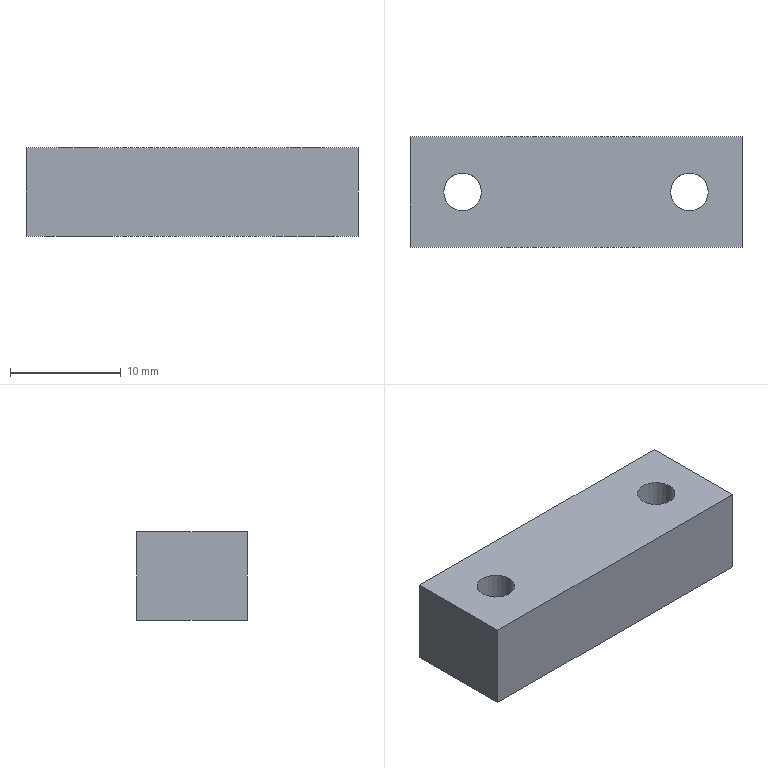Part | SolidWorks | features Extrusion 1, HoleWzd 1 | 1 solid | 16 faces | box 30 x 10 x 8 mm | volume 2124 mm3 | cylinder 8 | plane 8 | commonest cylinder face diameters 3.4 x4 6 x4
STEP:
#1=CARTESIAN_POINT('',(13.25,0.,3.4));
#2=VERTEX_POINT('',#1);
#3=CARTESIAN_POINT('',(7.25,0.,3.4));
#4=VERTEX_POINT('',#3);
#5=CARTESIAN_POINT('',(10.25,0.,3.4));
#6=DIRECTION('',(0.,0.,-1.));
#7=DIRECTION('',(-1.,0.,0.));
#8=AXIS2_PLACEMENT_3D('',#5,#6,#7);
#9=CIRCLE('',#8,3.);
#10=EDGE_CURVE('',#2,#4,#9,.T.);
#11=ORIENTED_EDGE('',*,*,#10,.F.);
#12=CARTESIAN_POINT('',(13.25,0.,0.));
#13=VERTEX_POINT('',#12);
#14=CARTESIAN_POINT('',(13.25,0.,0.));
#15=DIRECTION('',(0.,0.,-1.));
#16=VECTOR('',#15,1000.);
#17=LINE('',#14,#16);
#18=EDGE_CURVE('',#2,#13,#17,.T.);
#19=ORIENTED_EDGE('',*,*,#18,.T.);
#20=CARTESIAN_POINT('',(7.25,0.,0.));
#21=VERTEX_POINT('',#20);
#22=CARTESIAN_POINT('',(10.25,0.,0.));
#23=DIRECTION('',(0.,0.,-1.));
#24=DIRECTION('',(-1.,0.,0.));
#25=AXIS2_PLACEMENT_3D('',#22,#23,#24);
#26=CIRCLE('',#25,3.);
#27=EDGE_CURVE('',#13,#21,#26,.T.);
#28=ORIENTED_EDGE('',*,*,#27,.T.);
#29=CARTESIAN_POINT('',(7.25,0.,0.));
#30=DIRECTION('',(0.,0.,-1.));
#31=VECTOR('',#30,1000.);
#32=LINE('',#29,#31);
#33=EDGE_CURVE('',#4,#21,#32,.T.);
#34=ORIENTED_EDGE('',*,*,#33,.F.);
#35=EDGE_LOOP('',(#11,#19,#28,#34));
#36=FACE_OUTER_BOUND('',#35,.T.);
#37=CARTESIAN_POINT('',(10.25,0.,0.));
#38=DIRECTION('',(0.,0.,-1.));
#39=DIRECTION('',(-1.,0.,0.));
#40=AXIS2_PLACEMENT_3D('',#37,#38,#39);
#41=CYLINDRICAL_SURFACE('',#40,3.);
#42=ADVANCED_FACE('',(#36),#41,.F.);
#43=CARTESIAN_POINT('',(8.55,0.,8.));
#44=VERTEX_POINT('',#43);
#45=CARTESIAN_POINT('',(11.95,0.,8.));
#46=VERTEX_POINT('',#45);
#47=CARTESIAN_POINT('',(10.25,0.,8.));
#48=DIRECTION('',(0.,0.,1.));
#49=DIRECTION('',(1.,0.,0.));
#50=AXIS2_PLACEMENT_3D('',#47,#48,#49);
#51=CIRCLE('',#50,1.7);
#52=EDGE_CURVE('',#44,#46,#51,.T.);
#53=ORIENTED_EDGE('',*,*,#52,.T.);
#54=CARTESIAN_POINT('',(11.95,0.,3.4));
#55=VERTEX_POINT('',#54);
#56=CARTESIAN_POINT('',(11.95,0.,0.));
#57=DIRECTION('',(0.,0.,-1.));
#58=VECTOR('',#57,1000.);
#59=LINE('',#56,#58);
#60=EDGE_CURVE('',#46,#55,#59,.T.);
#61=ORIENTED_EDGE('',*,*,#60,.T.);
#62=CARTESIAN_POINT('',(8.55,0.,3.4));
#63=VERTEX_POINT('',#62);
#64=CARTESIAN_POINT('',(10.25,0.,3.4));
#65=DIRECTION('',(0.,0.,-1.));
#66=DIRECTION('',(-1.,0.,0.));
#67=AXIS2_PLACEMENT_3D('',#64,#65,#66);
#68=CIRCLE('',#67,1.7);
#69=EDGE_CURVE('',#55,#63,#68,.T.);
#70=ORIENTED_EDGE('',*,*,#69,.T.);
#71=CARTESIAN_POINT('',(8.55,0.,0.));
#72=DIRECTION('',(0.,0.,-1.));
#73=VECTOR('',#72,1000.);
#74=LINE('',#71,#73);
#75=EDGE_CURVE('',#44,#63,#74,.T.);
#76=ORIENTED_EDGE('',*,*,#75,.F.);
#77=EDGE_LOOP('',(#53,#61,#70,#76));
#78=FACE_OUTER_BOUND('',#77,.T.);
#79=CARTESIAN_POINT('',(10.25,0.,0.));
#80=DIRECTION('',(0.,0.,-1.));
#81=DIRECTION('',(-1.,0.,0.));
#82=AXIS2_PLACEMENT_3D('',#79,#80,#81);
#83=CYLINDRICAL_SURFACE('',#82,1.7);
#84=ADVANCED_FACE('',(#78),#83,.F.);
#85=CARTESIAN_POINT('',(-7.25,0.,3.4));
#86=VERTEX_POINT('',#85);
#87=CARTESIAN_POINT('',(-13.25,0.,3.4));
#88=VERTEX_POINT('',#87);
#89=CARTESIAN_POINT('',(-10.25,0.,3.4));
#90=DIRECTION('',(0.,0.,-1.));
#91=DIRECTION('',(-1.,0.,0.));
#92=AXIS2_PLACEMENT_3D('',#89,#90,#91);
#93=CIRCLE('',#92,3.);
#94=EDGE_CURVE('',#86,#88,#93,.T.);
#95=ORIENTED_EDGE('',*,*,#94,.F.);
#96=CARTESIAN_POINT('',(-7.25,0.,0.));
#97=VERTEX_POINT('',#96);
#98=CARTESIAN_POINT('',(-7.25,0.,0.));
#99=DIRECTION('',(0.,0.,-1.));
#100=VECTOR('',#99,1000.);
#101=LINE('',#98,#100);
#102=EDGE_CURVE('',#86,#97,#101,.T.);
#103=ORIENTED_EDGE('',*,*,#102,.T.);
#104=CARTESIAN_POINT('',(-13.25,0.,0.));
#105=VERTEX_POINT('',#104);
#106=CARTESIAN_POINT('',(-10.25,0.,0.));
#107=DIRECTION('',(0.,0.,-1.));
#108=DIRECTION('',(-1.,0.,0.));
#109=AXIS2_PLACEMENT_3D('',#106,#107,#108);
#110=CIRCLE('',#109,3.);
#111=EDGE_CURVE('',#97,#105,#110,.T.);
#112=ORIENTED_EDGE('',*,*,#111,.T.);
#113=CARTESIAN_POINT('',(-13.25,0.,0.));
#114=DIRECTION('',(0.,0.,-1.));
#115=VECTOR('',#114,1000.);
#116=LINE('',#113,#115);
#117=EDGE_CURVE('',#88,#105,#116,.T.);
#118=ORIENTED_EDGE('',*,*,#117,.F.);
#119=EDGE_LOOP('',(#95,#103,#112,#118));
#120=FACE_OUTER_BOUND('',#119,.T.);
#121=CARTESIAN_POINT('',(-10.25,0.,0.));
#122=DIRECTION('',(0.,0.,-1.));
#123=DIRECTION('',(-1.,0.,0.));
#124=AXIS2_PLACEMENT_3D('',#121,#122,#123);
#125=CYLINDRICAL_SURFACE('',#124,3.);
#126=ADVANCED_FACE('',(#120),#125,.F.);
#127=CARTESIAN_POINT('',(-11.95,0.,8.));
#128=VERTEX_POINT('',#127);
#129=CARTESIAN_POINT('',(-8.55,0.,8.));
#130=VERTEX_POINT('',#129);
#131=CARTESIAN_POINT('',(-10.25,0.,8.));
#132=DIRECTION('',(0.,0.,1.));
#133=DIRECTION('',(1.,0.,0.));
#134=AXIS2_PLACEMENT_3D('',#131,#132,#133);
#135=CIRCLE('',#134,1.7);
#136=EDGE_CURVE('',#128,#130,#135,.T.);
#137=ORIENTED_EDGE('',*,*,#136,.T.);
#138=CARTESIAN_POINT('',(-8.55,0.,3.4));
#139=VERTEX_POINT('',#138);
#140=CARTESIAN_POINT('',(-8.55,0.,0.));
#141=DIRECTION('',(0.,0.,-1.));
#142=VECTOR('',#141,1000.);
#143=LINE('',#140,#142);
#144=EDGE_CURVE('',#130,#139,#143,.T.);
#145=ORIENTED_EDGE('',*,*,#144,.T.);
#146=CARTESIAN_POINT('',(-11.95,0.,3.4));
#147=VERTEX_POINT('',#146);
#148=CARTESIAN_POINT('',(-10.25,0.,3.4));
#149=DIRECTION('',(0.,0.,-1.));
#150=DIRECTION('',(-1.,0.,0.));
#151=AXIS2_PLACEMENT_3D('',#148,#149,#150);
#152=CIRCLE('',#151,1.7);
#153=EDGE_CURVE('',#139,#147,#152,.T.);
#154=ORIENTED_EDGE('',*,*,#153,.T.);
#155=CARTESIAN_POINT('',(-11.95,0.,0.));
#156=DIRECTION('',(0.,0.,-1.));
#157=VECTOR('',#156,1000.);
#158=LINE('',#155,#157);
#159=EDGE_CURVE('',#128,#147,#158,.T.);
#160=ORIENTED_EDGE('',*,*,#159,.F.);
#161=EDGE_LOOP('',(#137,#145,#154,#160));
#162=FACE_OUTER_BOUND('',#161,.T.);
#163=CARTESIAN_POINT('',(-10.25,0.,0.));
#164=DIRECTION('',(0.,0.,-1.));
#165=DIRECTION('',(-1.,0.,0.));
#166=AXIS2_PLACEMENT_3D('',#163,#164,#165);
#167=CYLINDRICAL_SURFACE('',#166,1.7);
#168=ADVANCED_FACE('',(#162),#167,.F.);
#169=CARTESIAN_POINT('',(-15.,5.,0.));
#170=VERTEX_POINT('',#169);
#171=CARTESIAN_POINT('',(-15.,-5.,0.));
#172=VERTEX_POINT('',#171);
#173=CARTESIAN_POINT('',(-15.,-5.,0.));
#174=DIRECTION('',(0.,-1.,0.));
#175=VECTOR('',#174,1000.);
#176=LINE('',#173,#175);
#177=EDGE_CURVE('',#170,#172,#176,.T.);
#178=ORIENTED_EDGE('',*,*,#177,.T.);
#179=CARTESIAN_POINT('',(-15.,-5.,8.));
#180=VERTEX_POINT('',#179);
#181=CARTESIAN_POINT('',(-15.,-5.,8.));
#182=DIRECTION('',(0.,0.,-1.));
#183=VECTOR('',#182,1000.);
#184=LINE('',#181,#183);
#185=EDGE_CURVE('',#180,#172,#184,.T.);
#186=ORIENTED_EDGE('',*,*,#185,.F.);
#187=CARTESIAN_POINT('',(-15.,5.,8.));
#188=VERTEX_POINT('',#187);
#189=CARTESIAN_POINT('',(-15.,-5.,8.));
#190=DIRECTION('',(0.,-1.,0.));
#191=VECTOR('',#190,1000.);
#192=LINE('',#189,#191);
#193=EDGE_CURVE('',#188,#180,#192,.T.);
#194=ORIENTED_EDGE('',*,*,#193,.F.);
#195=CARTESIAN_POINT('',(-15.,5.,8.));
#196=DIRECTION('',(0.,0.,-1.));
#197=VECTOR('',#196,1000.);
#198=LINE('',#195,#197);
#199=EDGE_CURVE('',#188,#170,#198,.T.);
#200=ORIENTED_EDGE('',*,*,#199,.T.);
#201=EDGE_LOOP('',(#178,#186,#194,#200));
#202=FACE_OUTER_BOUND('',#201,.T.);
#203=CARTESIAN_POINT('',(-15.,-5.,8.));
#204=DIRECTION('',(1.,0.,0.));
#205=DIRECTION('',(0.,0.,-1.));
#206=AXIS2_PLACEMENT_3D('',#203,#204,#205);
#207=PLANE('',#206);
#208=ADVANCED_FACE('',(#202),#207,.F.);
#209=CARTESIAN_POINT('',(15.,-5.,0.));
#210=VERTEX_POINT('',#209);
#211=CARTESIAN_POINT('',(15.,-5.,0.));
#212=DIRECTION('',(1.,0.,0.));
#213=VECTOR('',#212,1000.);
#214=LINE('',#211,#213);
#215=EDGE_CURVE('',#172,#210,#214,.T.);
#216=ORIENTED_EDGE('',*,*,#215,.T.);
#217=CARTESIAN_POINT('',(15.,-5.,8.));
#218=VERTEX_POINT('',#217);
#219=CARTESIAN_POINT('',(15.,-5.,8.));
#220=DIRECTION('',(0.,0.,-1.));
#221=VECTOR('',#220,1000.);
#222=LINE('',#219,#221);
#223=EDGE_CURVE('',#218,#210,#222,.T.);
#224=ORIENTED_EDGE('',*,*,#223,.F.);
#225=CARTESIAN_POINT('',(15.,-5.,8.));
#226=DIRECTION('',(1.,0.,0.));
#227=VECTOR('',#226,1000.);
#228=LINE('',#225,#227);
#229=EDGE_CURVE('',#180,#218,#228,.T.);
#230=ORIENTED_EDGE('',*,*,#229,.F.);
#231=ORIENTED_EDGE('',*,*,#185,.T.);
#232=EDGE_LOOP('',(#216,#224,#230,#231));
#233=FACE_OUTER_BOUND('',#232,.T.);
#234=CARTESIAN_POINT('',(15.,-5.,8.));
#235=DIRECTION('',(0.,1.,0.));
#236=DIRECTION('',(-1.,0.,0.));
#237=AXIS2_PLACEMENT_3D('',#234,#235,#236);
#238=PLANE('',#237);
#239=ADVANCED_FACE('',(#233),#238,.F.);
#240=CARTESIAN_POINT('',(15.,5.,0.));
#241=VERTEX_POINT('',#240);
#242=CARTESIAN_POINT('',(15.,-5.,0.));
#243=DIRECTION('',(0.,1.,0.));
#244=VECTOR('',#243,1000.);
#245=LINE('',#242,#244);
#246=EDGE_CURVE('',#210,#241,#245,.T.);
#247=ORIENTED_EDGE('',*,*,#246,.T.);
#248=CARTESIAN_POINT('',(15.,5.,8.));
#249=VERTEX_POINT('',#248);
#250=CARTESIAN_POINT('',(15.,5.,8.));
#251=DIRECTION('',(0.,0.,-1.));
#252=VECTOR('',#251,1000.);
#253=LINE('',#250,#252);
#254=EDGE_CURVE('',#249,#241,#253,.T.);
#255=ORIENTED_EDGE('',*,*,#254,.F.);
#256=CARTESIAN_POINT('',(15.,-5.,8.));
#257=DIRECTION('',(0.,1.,0.));
#258=VECTOR('',#257,1000.);
#259=LINE('',#256,#258);
#260=EDGE_CURVE('',#218,#249,#259,.T.);
#261=ORIENTED_EDGE('',*,*,#260,.F.);
#262=ORIENTED_EDGE('',*,*,#223,.T.);
#263=EDGE_LOOP('',(#247,#255,#261,#262));
#264=FACE_OUTER_BOUND('',#263,.T.);
#265=CARTESIAN_POINT('',(15.,-5.,8.));
#266=DIRECTION('',(-1.,0.,0.));
#267=DIRECTION('',(0.,0.,1.));
#268=AXIS2_PLACEMENT_3D('',#265,#266,#267);
#269=PLANE('',#268);
#270=ADVANCED_FACE('',(#264),#269,.F.);
#271=CARTESIAN_POINT('',(15.,5.,0.));
#272=DIRECTION('',(-1.,0.,0.));
#273=VECTOR('',#272,1000.);
#274=LINE('',#271,#273);
#275=EDGE_CURVE('',#241,#170,#274,.T.);
#276=ORIENTED_EDGE('',*,*,#275,.T.);
#277=ORIENTED_EDGE('',*,*,#199,.F.);
#278=CARTESIAN_POINT('',(15.,5.,8.));
#279=DIRECTION('',(-1.,0.,0.));
#280=VECTOR('',#279,1000.);
#281=LINE('',#278,#280);
#282=EDGE_CURVE('',#249,#188,#281,.T.);
#283=ORIENTED_EDGE('',*,*,#282,.F.);
#284=ORIENTED_EDGE('',*,*,#254,.T.);
#285=EDGE_LOOP('',(#276,#277,#283,#284));
#286=FACE_OUTER_BOUND('',#285,.T.);
#287=CARTESIAN_POINT('',(15.,5.,8.));
#288=DIRECTION('',(0.,-1.,0.));
#289=DIRECTION('',(1.,0.,0.));
#290=AXIS2_PLACEMENT_3D('',#287,#288,#289);
#291=PLANE('',#290);
#292=ADVANCED_FACE('',(#286),#291,.F.);
#293=ORIENTED_EDGE('',*,*,#52,.F.);
#294=CARTESIAN_POINT('',(10.25,0.,8.));
#295=DIRECTION('',(0.,0.,1.));
#296=DIRECTION('',(1.,0.,0.));
#297=AXIS2_PLACEMENT_3D('',#294,#295,#296);
#298=CIRCLE('',#297,1.7);
#299=EDGE_CURVE('',#46,#44,#298,.T.);
#300=ORIENTED_EDGE('',*,*,#299,.F.);
#301=EDGE_LOOP('',(#293,#300));
#302=FACE_BOUND('',#301,.T.);
#303=ORIENTED_EDGE('',*,*,#136,.F.);
#304=CARTESIAN_POINT('',(-10.25,0.,8.));
#305=DIRECTION('',(0.,0.,1.));
#306=DIRECTION('',(1.,0.,0.));
#307=AXIS2_PLACEMENT_3D('',#304,#305,#306);
#308=CIRCLE('',#307,1.7);
#309=EDGE_CURVE('',#130,#128,#308,.T.);
#310=ORIENTED_EDGE('',*,*,#309,.F.);
#311=EDGE_LOOP('',(#303,#310));
#312=FACE_BOUND('',#311,.T.);
#313=ORIENTED_EDGE('',*,*,#193,.T.);
#314=ORIENTED_EDGE('',*,*,#229,.T.);
#315=ORIENTED_EDGE('',*,*,#260,.T.);
#316=ORIENTED_EDGE('',*,*,#282,.T.);
#317=EDGE_LOOP('',(#313,#314,#315,#316));
#318=FACE_OUTER_BOUND('',#317,.T.);
#319=CARTESIAN_POINT('',(0.,0.,8.));
#320=DIRECTION('',(0.,0.,1.));
#321=DIRECTION('',(1.,0.,0.));
#322=AXIS2_PLACEMENT_3D('',#319,#320,#321);
#323=PLANE('',#322);
#324=ADVANCED_FACE('',(#302,#312,#318),#323,.T.);
#325=CARTESIAN_POINT('',(10.25,0.,0.));
#326=DIRECTION('',(0.,0.,-1.));
#327=DIRECTION('',(-1.,0.,0.));
#328=AXIS2_PLACEMENT_3D('',#325,#326,#327);
#329=CIRCLE('',#328,3.);
#330=EDGE_CURVE('',#21,#13,#329,.T.);
#331=ORIENTED_EDGE('',*,*,#330,.F.);
#332=ORIENTED_EDGE('',*,*,#27,.F.);
#333=EDGE_LOOP('',(#331,#332));
#334=FACE_BOUND('',#333,.T.);
#335=CARTESIAN_POINT('',(-10.25,0.,0.));
#336=DIRECTION('',(0.,0.,-1.));
#337=DIRECTION('',(-1.,0.,0.));
#338=AXIS2_PLACEMENT_3D('',#335,#336,#337);
#339=CIRCLE('',#338,3.);
#340=EDGE_CURVE('',#105,#97,#339,.T.);
#341=ORIENTED_EDGE('',*,*,#340,.F.);
#342=ORIENTED_EDGE('',*,*,#111,.F.);
#343=EDGE_LOOP('',(#341,#342));
#344=FACE_BOUND('',#343,.T.);
#345=ORIENTED_EDGE('',*,*,#177,.F.);
#346=ORIENTED_EDGE('',*,*,#275,.F.);
#347=ORIENTED_EDGE('',*,*,#246,.F.);
#348=ORIENTED_EDGE('',*,*,#215,.F.);
#349=EDGE_LOOP('',(#345,#346,#347,#348));
#350=FACE_OUTER_BOUND('',#349,.T.);
#351=CARTESIAN_POINT('',(0.,0.,0.));
#352=DIRECTION('',(0.,0.,1.));
#353=DIRECTION('',(1.,0.,0.));
#354=AXIS2_PLACEMENT_3D('',#351,#352,#353);
#355=PLANE('',#354);
#356=ADVANCED_FACE('',(#334,#344,#350),#355,.F.);
#357=ORIENTED_EDGE('',*,*,#144,.F.);
#358=ORIENTED_EDGE('',*,*,#309,.T.);
#359=ORIENTED_EDGE('',*,*,#159,.T.);
#360=CARTESIAN_POINT('',(-10.25,0.,3.4));
#361=DIRECTION('',(0.,0.,-1.));
#362=DIRECTION('',(-1.,0.,0.));
#363=AXIS2_PLACEMENT_3D('',#360,#361,#362);
#364=CIRCLE('',#363,1.7);
#365=EDGE_CURVE('',#147,#139,#364,.T.);
#366=ORIENTED_EDGE('',*,*,#365,.T.);
#367=EDGE_LOOP('',(#357,#358,#359,#366));
#368=FACE_OUTER_BOUND('',#367,.T.);
#369=CARTESIAN_POINT('',(-10.25,0.,0.));
#370=DIRECTION('',(0.,0.,-1.));
#371=DIRECTION('',(-1.,0.,0.));
#372=AXIS2_PLACEMENT_3D('',#369,#370,#371);
#373=CYLINDRICAL_SURFACE('',#372,1.7);
#374=ADVANCED_FACE('',(#368),#373,.F.);
#375=ORIENTED_EDGE('',*,*,#365,.F.);
#376=ORIENTED_EDGE('',*,*,#153,.F.);
#377=EDGE_LOOP('',(#375,#376));
#378=FACE_BOUND('',#377,.T.);
#379=CARTESIAN_POINT('',(-10.25,0.,3.4));
#380=DIRECTION('',(0.,0.,-1.));
#381=DIRECTION('',(-1.,0.,0.));
#382=AXIS2_PLACEMENT_3D('',#379,#380,#381);
#383=CIRCLE('',#382,3.);
#384=EDGE_CURVE('',#88,#86,#383,.T.);
#385=ORIENTED_EDGE('',*,*,#384,.T.);
#386=ORIENTED_EDGE('',*,*,#94,.T.);
#387=EDGE_LOOP('',(#385,#386));
#388=FACE_OUTER_BOUND('',#387,.T.);
#389=CARTESIAN_POINT('',(-8.55,0.,3.4));
#390=DIRECTION('',(0.,0.,1.));
#391=DIRECTION('',(1.,0.,0.));
#392=AXIS2_PLACEMENT_3D('',#389,#390,#391);
#393=PLANE('',#392);
#394=ADVANCED_FACE('',(#378,#388),#393,.F.);
#395=ORIENTED_EDGE('',*,*,#102,.F.);
#396=ORIENTED_EDGE('',*,*,#384,.F.);
#397=ORIENTED_EDGE('',*,*,#117,.T.);
#398=ORIENTED_EDGE('',*,*,#340,.T.);
#399=EDGE_LOOP('',(#395,#396,#397,#398));
#400=FACE_OUTER_BOUND('',#399,.T.);
#401=CARTESIAN_POINT('',(-10.25,0.,0.));
#402=DIRECTION('',(0.,0.,-1.));
#403=DIRECTION('',(-1.,0.,0.));
#404=AXIS2_PLACEMENT_3D('',#401,#402,#403);
#405=CYLINDRICAL_SURFACE('',#404,3.);
#406=ADVANCED_FACE('',(#400),#405,.F.);
#407=ORIENTED_EDGE('',*,*,#60,.F.);
#408=ORIENTED_EDGE('',*,*,#299,.T.);
#409=ORIENTED_EDGE('',*,*,#75,.T.);
#410=CARTESIAN_POINT('',(10.25,0.,3.4));
#411=DIRECTION('',(0.,0.,-1.));
#412=DIRECTION('',(-1.,0.,0.));
#413=AXIS2_PLACEMENT_3D('',#410,#411,#412);
#414=CIRCLE('',#413,1.7);
#415=EDGE_CURVE('',#63,#55,#414,.T.);
#416=ORIENTED_EDGE('',*,*,#415,.T.);
#417=EDGE_LOOP('',(#407,#408,#409,#416));
#418=FACE_OUTER_BOUND('',#417,.T.);
#419=CARTESIAN_POINT('',(10.25,0.,0.));
#420=DIRECTION('',(0.,0.,-1.));
#421=DIRECTION('',(-1.,0.,0.));
#422=AXIS2_PLACEMENT_3D('',#419,#420,#421);
#423=CYLINDRICAL_SURFACE('',#422,1.7);
#424=ADVANCED_FACE('',(#418),#423,.F.);
#425=ORIENTED_EDGE('',*,*,#415,.F.);
#426=ORIENTED_EDGE('',*,*,#69,.F.);
#427=EDGE_LOOP('',(#425,#426));
#428=FACE_BOUND('',#427,.T.);
#429=CARTESIAN_POINT('',(10.25,0.,3.4));
#430=DIRECTION('',(0.,0.,-1.));
#431=DIRECTION('',(-1.,0.,0.));
#432=AXIS2_PLACEMENT_3D('',#429,#430,#431);
#433=CIRCLE('',#432,3.);
#434=EDGE_CURVE('',#4,#2,#433,.T.);
#435=ORIENTED_EDGE('',*,*,#434,.T.);
#436=ORIENTED_EDGE('',*,*,#10,.T.);
#437=EDGE_LOOP('',(#435,#436));
#438=FACE_OUTER_BOUND('',#437,.T.);
#439=CARTESIAN_POINT('',(11.95,0.,3.4));
#440=DIRECTION('',(0.,0.,1.));
#441=DIRECTION('',(1.,0.,0.));
#442=AXIS2_PLACEMENT_3D('',#439,#440,#441);
#443=PLANE('',#442);
#444=ADVANCED_FACE('',(#428,#438),#443,.F.);
#445=ORIENTED_EDGE('',*,*,#18,.F.);
#446=ORIENTED_EDGE('',*,*,#434,.F.);
#447=ORIENTED_EDGE('',*,*,#33,.T.);
#448=ORIENTED_EDGE('',*,*,#330,.T.);
#449=EDGE_LOOP('',(#445,#446,#447,#448));
#450=FACE_OUTER_BOUND('',#449,.T.);
#451=CARTESIAN_POINT('',(10.25,0.,0.));
#452=DIRECTION('',(0.,0.,-1.));
#453=DIRECTION('',(-1.,0.,0.));
#454=AXIS2_PLACEMENT_3D('',#451,#452,#453);
#455=CYLINDRICAL_SURFACE('',#454,3.);
#456=ADVANCED_FACE('',(#450),#455,.F.);
#457=CLOSED_SHELL('',(#42,#84,#126,#168,#208,#239,#270,#292,#324,#356,#374,#394,#406,#424,#444,#456));
#458=MANIFOLD_SOLID_BREP('',#457);
#459=CARTESIAN_POINT('',(0.,0.,0.));
#460=DIRECTION('',(0.,0.,1.));
#461=DIRECTION('',(1.,0.,0.));
#462=AXIS2_PLACEMENT_3D('',#459,#460,#461);
#463=(LENGTH_UNIT()NAMED_UNIT(*)SI_UNIT(.MILLI.,.METRE.));
#464=UNCERTAINTY_MEASURE_WITH_UNIT(LENGTH_MEASURE(0.00001),#463,'','');
#465=(NAMED_UNIT(*)PLANE_ANGLE_UNIT()SI_UNIT($,.RADIAN.));
#466=(NAMED_UNIT(*)SI_UNIT($,.STERADIAN.)SOLID_ANGLE_UNIT());
#467=(GEOMETRIC_REPRESENTATION_CONTEXT(3)GLOBAL_UNCERTAINTY_ASSIGNED_CONTEXT((#464))GLOBAL_UNIT_ASSIGNED_CONTEXT((#463,#465,#466))REPRESENTATION_CONTEXT('',''));
#468=ADVANCED_BREP_SHAPE_REPRESENTATION('',(#458,#462),#467);